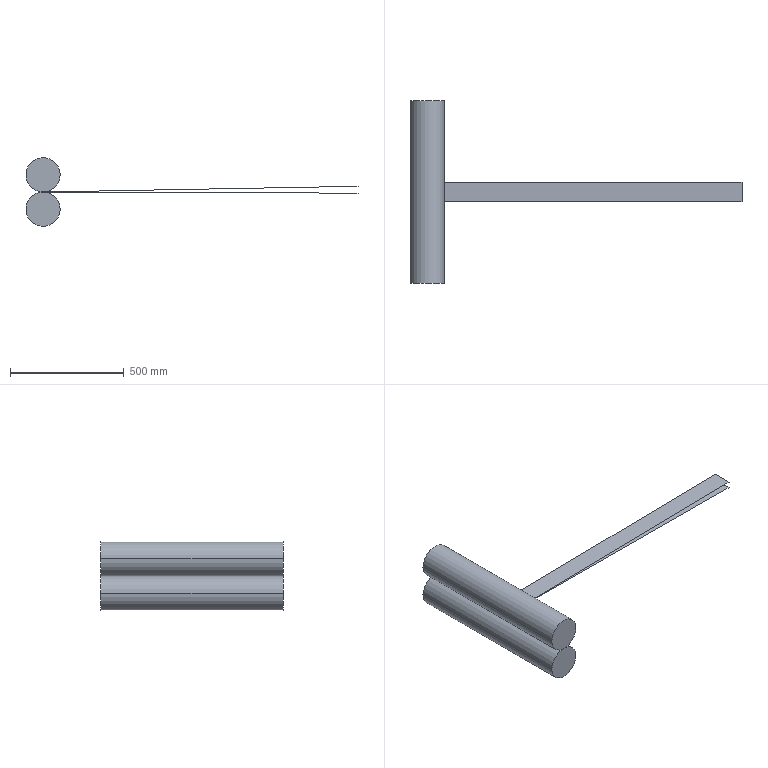Part | CATIA | 2 solids | 10 faces | box 1458 x 800 x 300 mm | volume 28421278 mm3 | plane 6 | cylinder 4 | commonest cylinder face diameters 150 x4